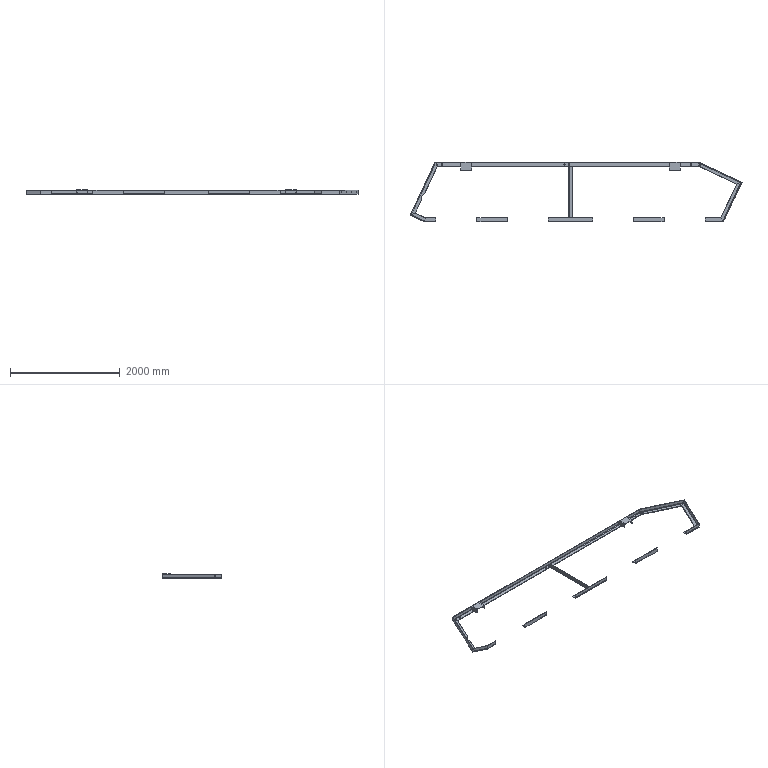Part | STEP file | Part 4_Default<As machined> | 13 solids | 175 faces | box 6040 x 1090 x 81 mm | volume 13497618 mm3 | plane 111 | cylinder 64 | commonest cylinder face diameters 5.333 x23 18 x19 22 x17 11 x4 224 x1